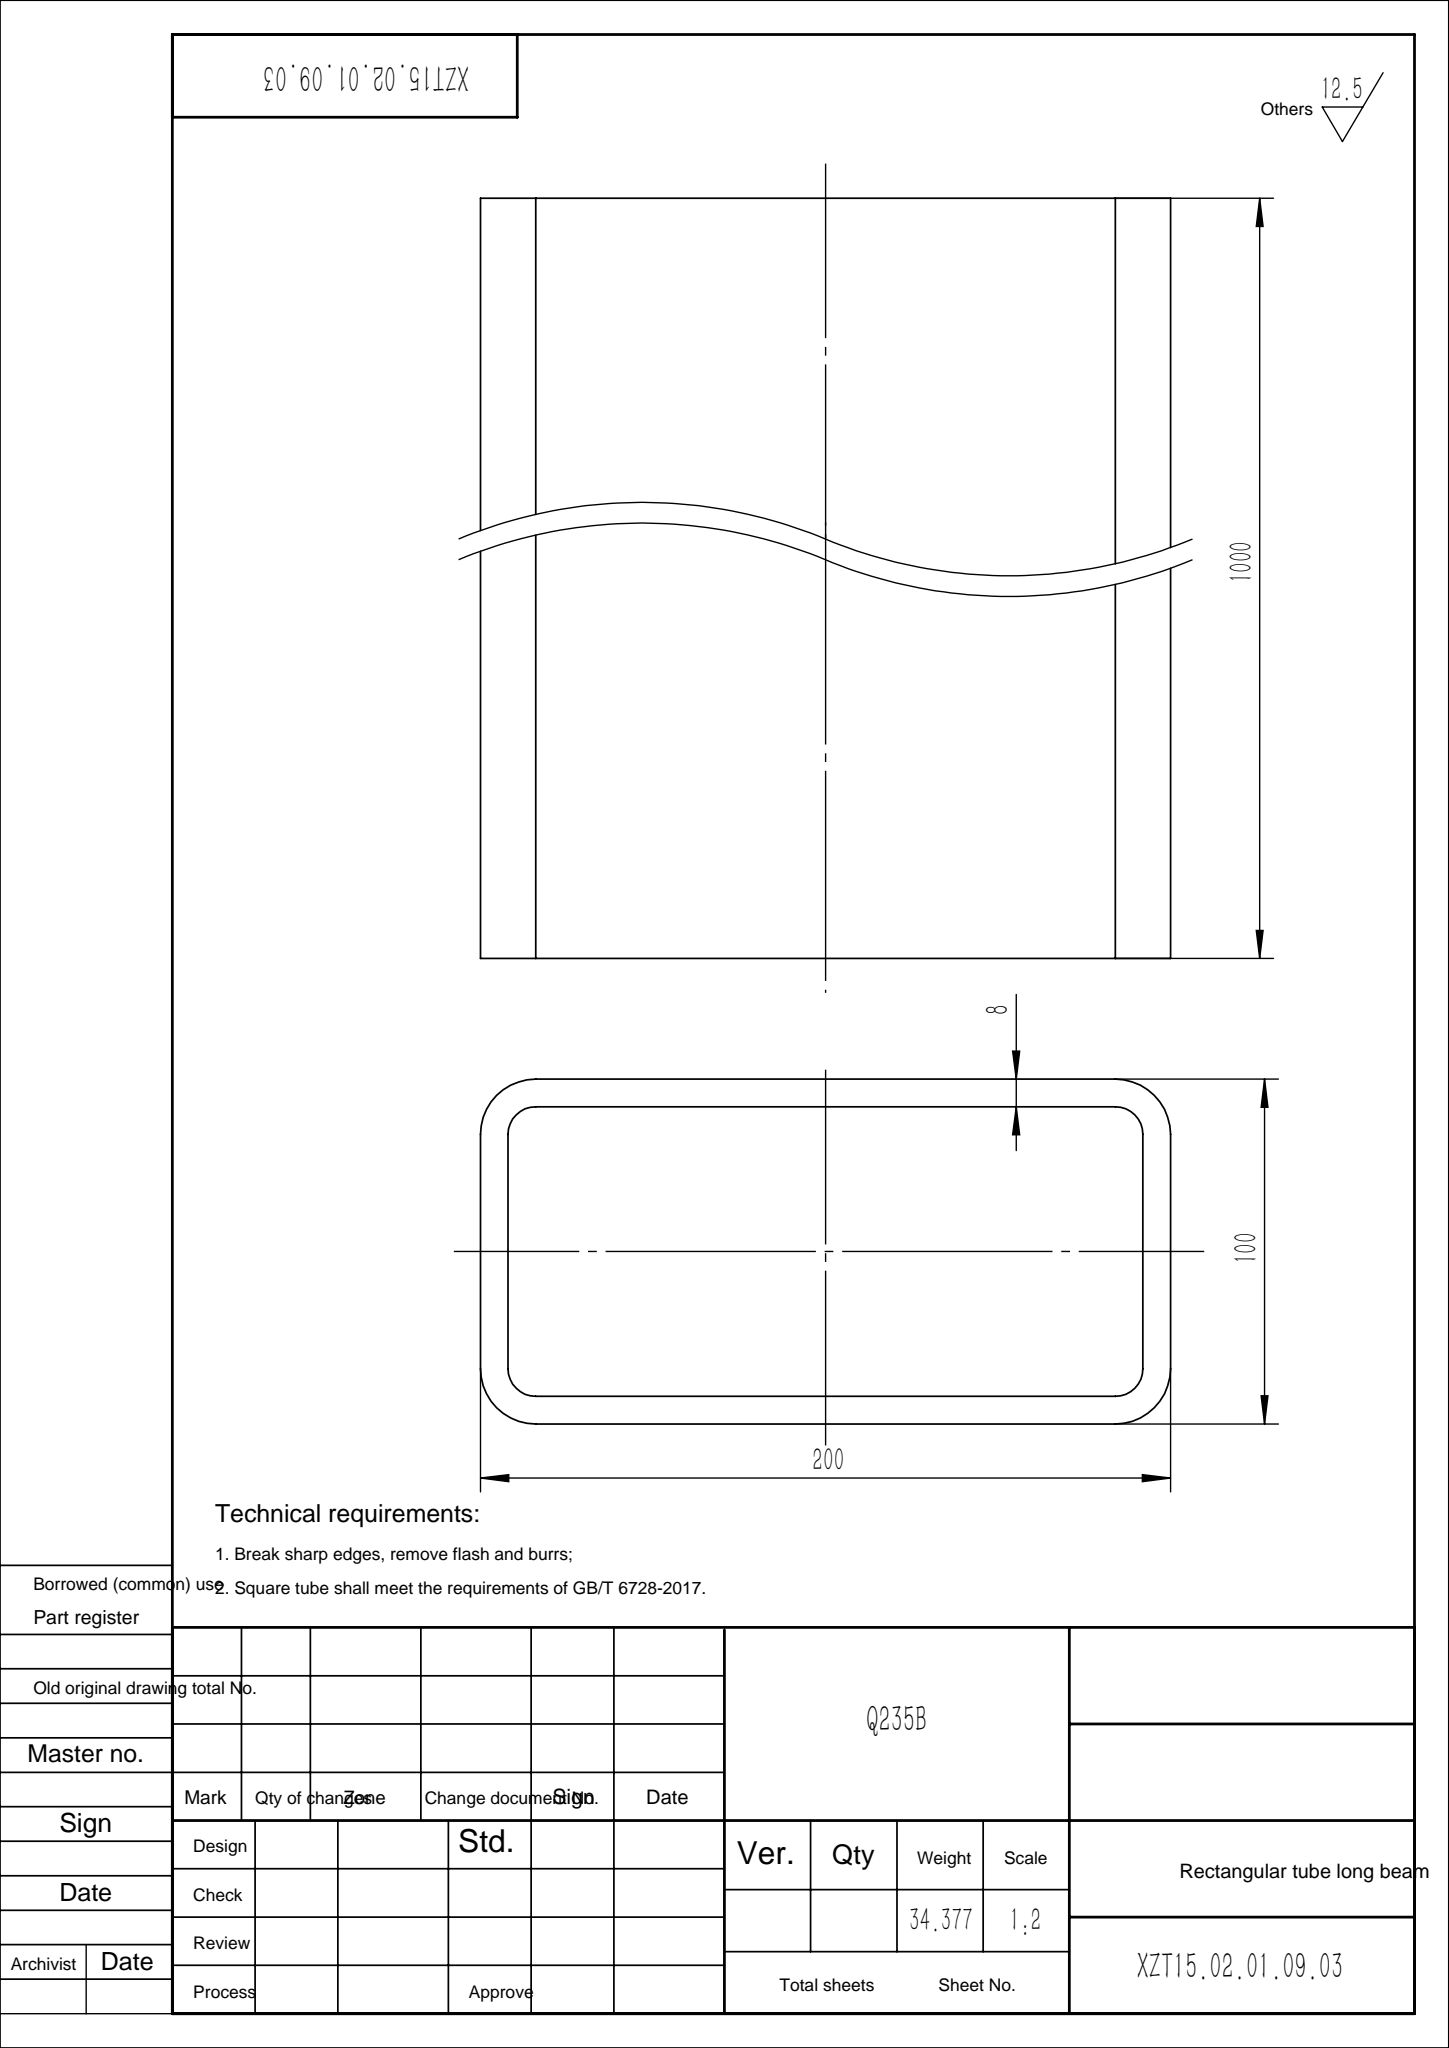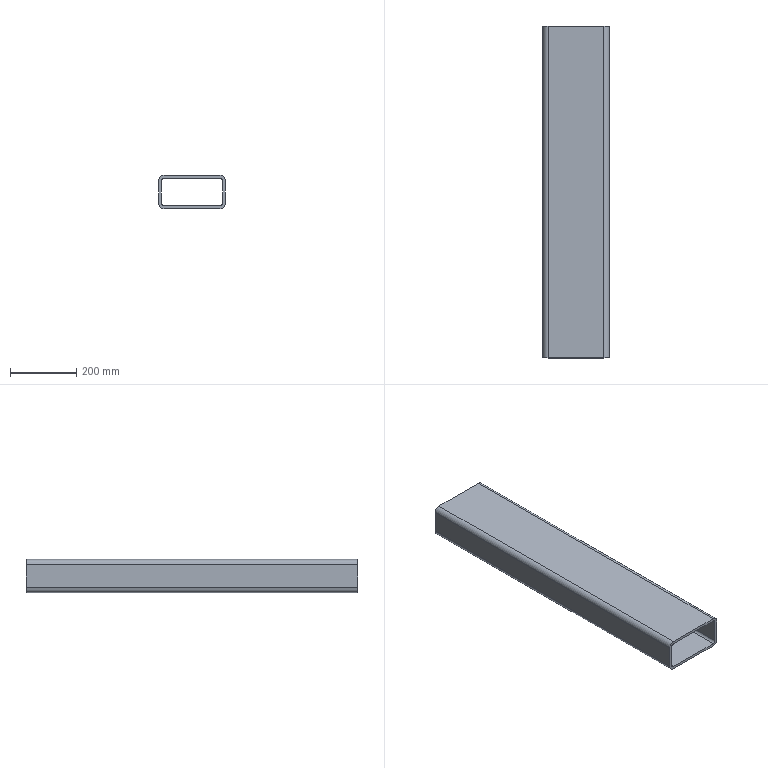Part | SolidWorks | features WeldMemberFeat 1, WeldmentFeature 1 | 1 solid | 18 faces | box 200 x 1000 x 100 mm | volume 4379186 mm3 | plane 10 | cylinder 8 | commonest cylinder face diameters 16 x4 32 x4
STEP:
#1=CARTESIAN_POINT('',(84.,0.,50.));
#2=VERTEX_POINT('',#1);
#3=CARTESIAN_POINT('',(100.,0.,34.));
#4=VERTEX_POINT('',#3);
#5=CARTESIAN_POINT('',(84.,0.,34.));
#6=DIRECTION('',(0.,1.,0.));
#7=DIRECTION('',(0.,0.,1.));
#8=AXIS2_PLACEMENT_3D('',#5,#6,#7);
#9=CIRCLE('',#8,16.);
#10=EDGE_CURVE('',#2,#4,#9,.T.);
#11=ORIENTED_EDGE('',*,*,#10,.T.);
#12=CARTESIAN_POINT('',(100.,1000.,34.));
#13=VERTEX_POINT('',#12);
#14=CARTESIAN_POINT('',(100.,1000.,34.));
#15=DIRECTION('',(0.,-1.,0.));
#16=VECTOR('',#15,1000.);
#17=LINE('',#14,#16);
#18=EDGE_CURVE('',#13,#4,#17,.T.);
#19=ORIENTED_EDGE('',*,*,#18,.F.);
#20=CARTESIAN_POINT('',(84.,1000.,50.));
#21=VERTEX_POINT('',#20);
#22=CARTESIAN_POINT('',(84.,1000.,34.));
#23=DIRECTION('',(0.,1.,0.));
#24=DIRECTION('',(0.,0.,1.));
#25=AXIS2_PLACEMENT_3D('',#22,#23,#24);
#26=CIRCLE('',#25,16.);
#27=EDGE_CURVE('',#21,#13,#26,.T.);
#28=ORIENTED_EDGE('',*,*,#27,.F.);
#29=CARTESIAN_POINT('',(84.,1000.,50.));
#30=DIRECTION('',(0.,-1.,0.));
#31=VECTOR('',#30,1000.);
#32=LINE('',#29,#31);
#33=EDGE_CURVE('',#21,#2,#32,.T.);
#34=ORIENTED_EDGE('',*,*,#33,.T.);
#35=EDGE_LOOP('',(#11,#19,#28,#34));
#36=FACE_OUTER_BOUND('',#35,.T.);
#37=CARTESIAN_POINT('',(84.,1000.,34.));
#38=DIRECTION('',(0.,-1.,0.));
#39=DIRECTION('',(0.,0.,-1.));
#40=AXIS2_PLACEMENT_3D('',#37,#38,#39);
#41=CYLINDRICAL_SURFACE('',#40,16.);
#42=ADVANCED_FACE('',(#36),#41,.T.);
#43=CARTESIAN_POINT('',(100.,0.,-34.));
#44=VERTEX_POINT('',#43);
#45=CARTESIAN_POINT('',(100.,0.,34.));
#46=DIRECTION('',(0.,0.,-1.));
#47=VECTOR('',#46,1000.);
#48=LINE('',#45,#47);
#49=EDGE_CURVE('',#4,#44,#48,.T.);
#50=ORIENTED_EDGE('',*,*,#49,.T.);
#51=CARTESIAN_POINT('',(100.,1000.,-34.));
#52=VERTEX_POINT('',#51);
#53=CARTESIAN_POINT('',(100.,1000.,-34.));
#54=DIRECTION('',(0.,-1.,0.));
#55=VECTOR('',#54,1000.);
#56=LINE('',#53,#55);
#57=EDGE_CURVE('',#52,#44,#56,.T.);
#58=ORIENTED_EDGE('',*,*,#57,.F.);
#59=CARTESIAN_POINT('',(100.,1000.,34.));
#60=DIRECTION('',(0.,0.,-1.));
#61=VECTOR('',#60,1000.);
#62=LINE('',#59,#61);
#63=EDGE_CURVE('',#13,#52,#62,.T.);
#64=ORIENTED_EDGE('',*,*,#63,.F.);
#65=ORIENTED_EDGE('',*,*,#18,.T.);
#66=EDGE_LOOP('',(#50,#58,#64,#65));
#67=FACE_OUTER_BOUND('',#66,.T.);
#68=CARTESIAN_POINT('',(100.,1000.,34.));
#69=DIRECTION('',(-1.,0.,0.));
#70=DIRECTION('',(0.,0.,1.));
#71=AXIS2_PLACEMENT_3D('',#68,#69,#70);
#72=PLANE('',#71);
#73=ADVANCED_FACE('',(#67),#72,.F.);
#74=CARTESIAN_POINT('',(84.,0.,-50.));
#75=VERTEX_POINT('',#74);
#76=CARTESIAN_POINT('',(84.,0.,-34.));
#77=DIRECTION('',(0.,1.,0.));
#78=DIRECTION('',(0.,0.,1.));
#79=AXIS2_PLACEMENT_3D('',#76,#77,#78);
#80=CIRCLE('',#79,16.);
#81=EDGE_CURVE('',#44,#75,#80,.T.);
#82=ORIENTED_EDGE('',*,*,#81,.T.);
#83=CARTESIAN_POINT('',(84.,1000.,-50.));
#84=VERTEX_POINT('',#83);
#85=CARTESIAN_POINT('',(84.,1000.,-50.));
#86=DIRECTION('',(0.,-1.,0.));
#87=VECTOR('',#86,1000.);
#88=LINE('',#85,#87);
#89=EDGE_CURVE('',#84,#75,#88,.T.);
#90=ORIENTED_EDGE('',*,*,#89,.F.);
#91=CARTESIAN_POINT('',(84.,1000.,-34.));
#92=DIRECTION('',(0.,1.,0.));
#93=DIRECTION('',(0.,0.,1.));
#94=AXIS2_PLACEMENT_3D('',#91,#92,#93);
#95=CIRCLE('',#94,16.);
#96=EDGE_CURVE('',#52,#84,#95,.T.);
#97=ORIENTED_EDGE('',*,*,#96,.F.);
#98=ORIENTED_EDGE('',*,*,#57,.T.);
#99=EDGE_LOOP('',(#82,#90,#97,#98));
#100=FACE_OUTER_BOUND('',#99,.T.);
#101=CARTESIAN_POINT('',(84.,1000.,-34.));
#102=DIRECTION('',(0.,-1.,0.));
#103=DIRECTION('',(0.,0.,-1.));
#104=AXIS2_PLACEMENT_3D('',#101,#102,#103);
#105=CYLINDRICAL_SURFACE('',#104,16.);
#106=ADVANCED_FACE('',(#100),#105,.T.);
#107=CARTESIAN_POINT('',(-84.,0.,-50.));
#108=VERTEX_POINT('',#107);
#109=CARTESIAN_POINT('',(-84.,0.,-50.));
#110=DIRECTION('',(-1.,0.,0.));
#111=VECTOR('',#110,1000.);
#112=LINE('',#109,#111);
#113=EDGE_CURVE('',#75,#108,#112,.T.);
#114=ORIENTED_EDGE('',*,*,#113,.T.);
#115=CARTESIAN_POINT('',(-84.,1000.,-50.));
#116=VERTEX_POINT('',#115);
#117=CARTESIAN_POINT('',(-84.,1000.,-50.));
#118=DIRECTION('',(0.,-1.,0.));
#119=VECTOR('',#118,1000.);
#120=LINE('',#117,#119);
#121=EDGE_CURVE('',#116,#108,#120,.T.);
#122=ORIENTED_EDGE('',*,*,#121,.F.);
#123=CARTESIAN_POINT('',(-84.,1000.,-50.));
#124=DIRECTION('',(-1.,0.,0.));
#125=VECTOR('',#124,1000.);
#126=LINE('',#123,#125);
#127=EDGE_CURVE('',#84,#116,#126,.T.);
#128=ORIENTED_EDGE('',*,*,#127,.F.);
#129=ORIENTED_EDGE('',*,*,#89,.T.);
#130=EDGE_LOOP('',(#114,#122,#128,#129));
#131=FACE_OUTER_BOUND('',#130,.T.);
#132=CARTESIAN_POINT('',(-84.,1000.,-50.));
#133=DIRECTION('',(0.,0.,1.));
#134=DIRECTION('',(1.,0.,0.));
#135=AXIS2_PLACEMENT_3D('',#132,#133,#134);
#136=PLANE('',#135);
#137=ADVANCED_FACE('',(#131),#136,.F.);
#138=CARTESIAN_POINT('',(-100.,0.,-34.));
#139=VERTEX_POINT('',#138);
#140=CARTESIAN_POINT('',(-84.,0.,-34.));
#141=DIRECTION('',(0.,1.,0.));
#142=DIRECTION('',(0.,0.,1.));
#143=AXIS2_PLACEMENT_3D('',#140,#141,#142);
#144=CIRCLE('',#143,16.);
#145=EDGE_CURVE('',#108,#139,#144,.T.);
#146=ORIENTED_EDGE('',*,*,#145,.T.);
#147=CARTESIAN_POINT('',(-100.,1000.,-34.));
#148=VERTEX_POINT('',#147);
#149=CARTESIAN_POINT('',(-100.,1000.,-34.));
#150=DIRECTION('',(0.,-1.,0.));
#151=VECTOR('',#150,1000.);
#152=LINE('',#149,#151);
#153=EDGE_CURVE('',#148,#139,#152,.T.);
#154=ORIENTED_EDGE('',*,*,#153,.F.);
#155=CARTESIAN_POINT('',(-84.,1000.,-34.));
#156=DIRECTION('',(0.,1.,0.));
#157=DIRECTION('',(0.,0.,1.));
#158=AXIS2_PLACEMENT_3D('',#155,#156,#157);
#159=CIRCLE('',#158,16.);
#160=EDGE_CURVE('',#116,#148,#159,.T.);
#161=ORIENTED_EDGE('',*,*,#160,.F.);
#162=ORIENTED_EDGE('',*,*,#121,.T.);
#163=EDGE_LOOP('',(#146,#154,#161,#162));
#164=FACE_OUTER_BOUND('',#163,.T.);
#165=CARTESIAN_POINT('',(-84.,1000.,-34.));
#166=DIRECTION('',(0.,-1.,0.));
#167=DIRECTION('',(0.,0.,-1.));
#168=AXIS2_PLACEMENT_3D('',#165,#166,#167);
#169=CYLINDRICAL_SURFACE('',#168,16.);
#170=ADVANCED_FACE('',(#164),#169,.T.);
#171=CARTESIAN_POINT('',(-100.,0.,34.));
#172=VERTEX_POINT('',#171);
#173=CARTESIAN_POINT('',(-100.,0.,-34.));
#174=DIRECTION('',(0.,0.,1.));
#175=VECTOR('',#174,1000.);
#176=LINE('',#173,#175);
#177=EDGE_CURVE('',#139,#172,#176,.T.);
#178=ORIENTED_EDGE('',*,*,#177,.T.);
#179=CARTESIAN_POINT('',(-100.,1000.,34.));
#180=VERTEX_POINT('',#179);
#181=CARTESIAN_POINT('',(-100.,1000.,34.));
#182=DIRECTION('',(0.,-1.,0.));
#183=VECTOR('',#182,1000.);
#184=LINE('',#181,#183);
#185=EDGE_CURVE('',#180,#172,#184,.T.);
#186=ORIENTED_EDGE('',*,*,#185,.F.);
#187=CARTESIAN_POINT('',(-100.,1000.,-34.));
#188=DIRECTION('',(0.,0.,1.));
#189=VECTOR('',#188,1000.);
#190=LINE('',#187,#189);
#191=EDGE_CURVE('',#148,#180,#190,.T.);
#192=ORIENTED_EDGE('',*,*,#191,.F.);
#193=ORIENTED_EDGE('',*,*,#153,.T.);
#194=EDGE_LOOP('',(#178,#186,#192,#193));
#195=FACE_OUTER_BOUND('',#194,.T.);
#196=CARTESIAN_POINT('',(-100.,1000.,-34.));
#197=DIRECTION('',(1.,0.,0.));
#198=DIRECTION('',(0.,0.,-1.));
#199=AXIS2_PLACEMENT_3D('',#196,#197,#198);
#200=PLANE('',#199);
#201=ADVANCED_FACE('',(#195),#200,.F.);
#202=CARTESIAN_POINT('',(-84.,0.,50.));
#203=VERTEX_POINT('',#202);
#204=CARTESIAN_POINT('',(-84.,0.,34.));
#205=DIRECTION('',(0.,1.,0.));
#206=DIRECTION('',(0.,0.,1.));
#207=AXIS2_PLACEMENT_3D('',#204,#205,#206);
#208=CIRCLE('',#207,16.);
#209=EDGE_CURVE('',#172,#203,#208,.T.);
#210=ORIENTED_EDGE('',*,*,#209,.T.);
#211=CARTESIAN_POINT('',(-84.,1000.,50.));
#212=VERTEX_POINT('',#211);
#213=CARTESIAN_POINT('',(-84.,1000.,50.));
#214=DIRECTION('',(0.,-1.,0.));
#215=VECTOR('',#214,1000.);
#216=LINE('',#213,#215);
#217=EDGE_CURVE('',#212,#203,#216,.T.);
#218=ORIENTED_EDGE('',*,*,#217,.F.);
#219=CARTESIAN_POINT('',(-84.,1000.,34.));
#220=DIRECTION('',(0.,1.,0.));
#221=DIRECTION('',(0.,0.,1.));
#222=AXIS2_PLACEMENT_3D('',#219,#220,#221);
#223=CIRCLE('',#222,16.);
#224=EDGE_CURVE('',#180,#212,#223,.T.);
#225=ORIENTED_EDGE('',*,*,#224,.F.);
#226=ORIENTED_EDGE('',*,*,#185,.T.);
#227=EDGE_LOOP('',(#210,#218,#225,#226));
#228=FACE_OUTER_BOUND('',#227,.T.);
#229=CARTESIAN_POINT('',(-84.,1000.,34.));
#230=DIRECTION('',(0.,-1.,0.));
#231=DIRECTION('',(0.,0.,-1.));
#232=AXIS2_PLACEMENT_3D('',#229,#230,#231);
#233=CYLINDRICAL_SURFACE('',#232,16.);
#234=ADVANCED_FACE('',(#228),#233,.T.);
#235=CARTESIAN_POINT('',(92.,0.,-34.));
#236=VERTEX_POINT('',#235);
#237=CARTESIAN_POINT('',(84.,0.,-42.));
#238=VERTEX_POINT('',#237);
#239=CARTESIAN_POINT('',(84.,0.,-34.));
#240=DIRECTION('',(0.,1.,0.));
#241=DIRECTION('',(0.,0.,1.));
#242=AXIS2_PLACEMENT_3D('',#239,#240,#241);
#243=CIRCLE('',#242,8.);
#244=EDGE_CURVE('',#236,#238,#243,.T.);
#245=ORIENTED_EDGE('',*,*,#244,.F.);
#246=CARTESIAN_POINT('',(92.,1000.,-34.));
#247=VERTEX_POINT('',#246);
#248=CARTESIAN_POINT('',(92.,1000.,-34.));
#249=DIRECTION('',(0.,-1.,0.));
#250=VECTOR('',#249,1000.);
#251=LINE('',#248,#250);
#252=EDGE_CURVE('',#247,#236,#251,.T.);
#253=ORIENTED_EDGE('',*,*,#252,.F.);
#254=CARTESIAN_POINT('',(84.,1000.,-42.));
#255=VERTEX_POINT('',#254);
#256=CARTESIAN_POINT('',(84.,1000.,-34.));
#257=DIRECTION('',(0.,1.,0.));
#258=DIRECTION('',(0.,0.,1.));
#259=AXIS2_PLACEMENT_3D('',#256,#257,#258);
#260=CIRCLE('',#259,8.);
#261=EDGE_CURVE('',#247,#255,#260,.T.);
#262=ORIENTED_EDGE('',*,*,#261,.T.);
#263=CARTESIAN_POINT('',(84.,1000.,-42.));
#264=DIRECTION('',(0.,-1.,0.));
#265=VECTOR('',#264,1000.);
#266=LINE('',#263,#265);
#267=EDGE_CURVE('',#255,#238,#266,.T.);
#268=ORIENTED_EDGE('',*,*,#267,.T.);
#269=EDGE_LOOP('',(#245,#253,#262,#268));
#270=FACE_OUTER_BOUND('',#269,.T.);
#271=CARTESIAN_POINT('',(84.,1000.,-34.));
#272=DIRECTION('',(0.,-1.,0.));
#273=DIRECTION('',(0.,0.,-1.));
#274=AXIS2_PLACEMENT_3D('',#271,#272,#273);
#275=CYLINDRICAL_SURFACE('',#274,8.);
#276=ADVANCED_FACE('',(#270),#275,.F.);
#277=CARTESIAN_POINT('',(92.,0.,34.));
#278=VERTEX_POINT('',#277);
#279=CARTESIAN_POINT('',(92.,0.,34.));
#280=DIRECTION('',(0.,0.,-1.));
#281=VECTOR('',#280,1000.);
#282=LINE('',#279,#281);
#283=EDGE_CURVE('',#278,#236,#282,.T.);
#284=ORIENTED_EDGE('',*,*,#283,.F.);
#285=CARTESIAN_POINT('',(92.,1000.,34.));
#286=VERTEX_POINT('',#285);
#287=CARTESIAN_POINT('',(92.,1000.,34.));
#288=DIRECTION('',(0.,-1.,0.));
#289=VECTOR('',#288,1000.);
#290=LINE('',#287,#289);
#291=EDGE_CURVE('',#286,#278,#290,.T.);
#292=ORIENTED_EDGE('',*,*,#291,.F.);
#293=CARTESIAN_POINT('',(92.,1000.,34.));
#294=DIRECTION('',(0.,0.,-1.));
#295=VECTOR('',#294,1000.);
#296=LINE('',#293,#295);
#297=EDGE_CURVE('',#286,#247,#296,.T.);
#298=ORIENTED_EDGE('',*,*,#297,.T.);
#299=ORIENTED_EDGE('',*,*,#252,.T.);
#300=EDGE_LOOP('',(#284,#292,#298,#299));
#301=FACE_OUTER_BOUND('',#300,.T.);
#302=CARTESIAN_POINT('',(92.,1000.,34.));
#303=DIRECTION('',(-1.,0.,0.));
#304=DIRECTION('',(0.,0.,1.));
#305=AXIS2_PLACEMENT_3D('',#302,#303,#304);
#306=PLANE('',#305);
#307=ADVANCED_FACE('',(#301),#306,.T.);
#308=CARTESIAN_POINT('',(84.,0.,42.));
#309=VERTEX_POINT('',#308);
#310=CARTESIAN_POINT('',(84.,0.,34.));
#311=DIRECTION('',(0.,1.,0.));
#312=DIRECTION('',(0.,0.,1.));
#313=AXIS2_PLACEMENT_3D('',#310,#311,#312);
#314=CIRCLE('',#313,8.);
#315=EDGE_CURVE('',#309,#278,#314,.T.);
#316=ORIENTED_EDGE('',*,*,#315,.F.);
#317=CARTESIAN_POINT('',(84.,1000.,42.));
#318=VERTEX_POINT('',#317);
#319=CARTESIAN_POINT('',(84.,1000.,42.));
#320=DIRECTION('',(0.,-1.,0.));
#321=VECTOR('',#320,1000.);
#322=LINE('',#319,#321);
#323=EDGE_CURVE('',#318,#309,#322,.T.);
#324=ORIENTED_EDGE('',*,*,#323,.F.);
#325=CARTESIAN_POINT('',(84.,1000.,34.));
#326=DIRECTION('',(0.,1.,0.));
#327=DIRECTION('',(0.,0.,1.));
#328=AXIS2_PLACEMENT_3D('',#325,#326,#327);
#329=CIRCLE('',#328,8.);
#330=EDGE_CURVE('',#318,#286,#329,.T.);
#331=ORIENTED_EDGE('',*,*,#330,.T.);
#332=ORIENTED_EDGE('',*,*,#291,.T.);
#333=EDGE_LOOP('',(#316,#324,#331,#332));
#334=FACE_OUTER_BOUND('',#333,.T.);
#335=CARTESIAN_POINT('',(84.,1000.,34.));
#336=DIRECTION('',(0.,-1.,0.));
#337=DIRECTION('',(0.,0.,-1.));
#338=AXIS2_PLACEMENT_3D('',#335,#336,#337);
#339=CYLINDRICAL_SURFACE('',#338,8.);
#340=ADVANCED_FACE('',(#334),#339,.F.);
#341=CARTESIAN_POINT('',(-84.,0.,42.));
#342=VERTEX_POINT('',#341);
#343=CARTESIAN_POINT('',(84.,0.,42.));
#344=DIRECTION('',(1.,0.,0.));
#345=VECTOR('',#344,1000.);
#346=LINE('',#343,#345);
#347=EDGE_CURVE('',#342,#309,#346,.T.);
#348=ORIENTED_EDGE('',*,*,#347,.F.);
#349=CARTESIAN_POINT('',(-84.,1000.,42.));
#350=VERTEX_POINT('',#349);
#351=CARTESIAN_POINT('',(-84.,1000.,42.));
#352=DIRECTION('',(0.,-1.,0.));
#353=VECTOR('',#352,1000.);
#354=LINE('',#351,#353);
#355=EDGE_CURVE('',#350,#342,#354,.T.);
#356=ORIENTED_EDGE('',*,*,#355,.F.);
#357=CARTESIAN_POINT('',(84.,1000.,42.));
#358=DIRECTION('',(1.,0.,0.));
#359=VECTOR('',#358,1000.);
#360=LINE('',#357,#359);
#361=EDGE_CURVE('',#350,#318,#360,.T.);
#362=ORIENTED_EDGE('',*,*,#361,.T.);
#363=ORIENTED_EDGE('',*,*,#323,.T.);
#364=EDGE_LOOP('',(#348,#356,#362,#363));
#365=FACE_OUTER_BOUND('',#364,.T.);
#366=CARTESIAN_POINT('',(84.,1000.,42.));
#367=DIRECTION('',(0.,0.,-1.));
#368=DIRECTION('',(-1.,0.,0.));
#369=AXIS2_PLACEMENT_3D('',#366,#367,#368);
#370=PLANE('',#369);
#371=ADVANCED_FACE('',(#365),#370,.T.);
#372=CARTESIAN_POINT('',(-92.,0.,34.));
#373=VERTEX_POINT('',#372);
#374=CARTESIAN_POINT('',(-84.,0.,34.));
#375=DIRECTION('',(0.,1.,0.));
#376=DIRECTION('',(0.,0.,1.));
#377=AXIS2_PLACEMENT_3D('',#374,#375,#376);
#378=CIRCLE('',#377,8.);
#379=EDGE_CURVE('',#373,#342,#378,.T.);
#380=ORIENTED_EDGE('',*,*,#379,.F.);
#381=CARTESIAN_POINT('',(-92.,1000.,34.));
#382=VERTEX_POINT('',#381);
#383=CARTESIAN_POINT('',(-92.,1000.,34.));
#384=DIRECTION('',(0.,-1.,0.));
#385=VECTOR('',#384,1000.);
#386=LINE('',#383,#385);
#387=EDGE_CURVE('',#382,#373,#386,.T.);
#388=ORIENTED_EDGE('',*,*,#387,.F.);
#389=CARTESIAN_POINT('',(-84.,1000.,34.));
#390=DIRECTION('',(0.,1.,0.));
#391=DIRECTION('',(0.,0.,1.));
#392=AXIS2_PLACEMENT_3D('',#389,#390,#391);
#393=CIRCLE('',#392,8.);
#394=EDGE_CURVE('',#382,#350,#393,.T.);
#395=ORIENTED_EDGE('',*,*,#394,.T.);
#396=ORIENTED_EDGE('',*,*,#355,.T.);
#397=EDGE_LOOP('',(#380,#388,#395,#396));
#398=FACE_OUTER_BOUND('',#397,.T.);
#399=CARTESIAN_POINT('',(-84.,1000.,34.));
#400=DIRECTION('',(0.,-1.,0.));
#401=DIRECTION('',(0.,0.,-1.));
#402=AXIS2_PLACEMENT_3D('',#399,#400,#401);
#403=CYLINDRICAL_SURFACE('',#402,8.);
#404=ADVANCED_FACE('',(#398),#403,.F.);
#405=CARTESIAN_POINT('',(-92.,0.,-34.));
#406=VERTEX_POINT('',#405);
#407=CARTESIAN_POINT('',(-92.,0.,-34.));
#408=DIRECTION('',(0.,0.,1.));
#409=VECTOR('',#408,1000.);
#410=LINE('',#407,#409);
#411=EDGE_CURVE('',#406,#373,#410,.T.);
#412=ORIENTED_EDGE('',*,*,#411,.F.);
#413=CARTESIAN_POINT('',(-92.,1000.,-34.));
#414=VERTEX_POINT('',#413);
#415=CARTESIAN_POINT('',(-92.,1000.,-34.));
#416=DIRECTION('',(0.,-1.,0.));
#417=VECTOR('',#416,1000.);
#418=LINE('',#415,#417);
#419=EDGE_CURVE('',#414,#406,#418,.T.);
#420=ORIENTED_EDGE('',*,*,#419,.F.);
#421=CARTESIAN_POINT('',(-92.,1000.,-34.));
#422=DIRECTION('',(0.,0.,1.));
#423=VECTOR('',#422,1000.);
#424=LINE('',#421,#423);
#425=EDGE_CURVE('',#414,#382,#424,.T.);
#426=ORIENTED_EDGE('',*,*,#425,.T.);
#427=ORIENTED_EDGE('',*,*,#387,.T.);
#428=EDGE_LOOP('',(#412,#420,#426,#427));
#429=FACE_OUTER_BOUND('',#428,.T.);
#430=CARTESIAN_POINT('',(-92.,1000.,-34.));
#431=DIRECTION('',(1.,0.,0.));
#432=DIRECTION('',(0.,0.,-1.));
#433=AXIS2_PLACEMENT_3D('',#430,#431,#432);
#434=PLANE('',#433);
#435=ADVANCED_FACE('',(#429),#434,.T.);
#436=CARTESIAN_POINT('',(-84.,0.,-42.));
#437=VERTEX_POINT('',#436);
#438=CARTESIAN_POINT('',(-84.,0.,-34.));
#439=DIRECTION('',(0.,1.,0.));
#440=DIRECTION('',(0.,0.,1.));
#441=AXIS2_PLACEMENT_3D('',#438,#439,#440);
#442=CIRCLE('',#441,8.);
#443=EDGE_CURVE('',#437,#406,#442,.T.);
#444=ORIENTED_EDGE('',*,*,#443,.F.);
#445=CARTESIAN_POINT('',(-84.,1000.,-42.));
#446=VERTEX_POINT('',#445);
#447=CARTESIAN_POINT('',(-84.,1000.,-42.));
#448=DIRECTION('',(0.,-1.,0.));
#449=VECTOR('',#448,1000.);
#450=LINE('',#447,#449);
#451=EDGE_CURVE('',#446,#437,#450,.T.);
#452=ORIENTED_EDGE('',*,*,#451,.F.);
#453=CARTESIAN_POINT('',(-84.,1000.,-34.));
#454=DIRECTION('',(0.,1.,0.));
#455=DIRECTION('',(0.,0.,1.));
#456=AXIS2_PLACEMENT_3D('',#453,#454,#455);
#457=CIRCLE('',#456,8.);
#458=EDGE_CURVE('',#446,#414,#457,.T.);
#459=ORIENTED_EDGE('',*,*,#458,.T.);
#460=ORIENTED_EDGE('',*,*,#419,.T.);
#461=EDGE_LOOP('',(#444,#452,#459,#460));
#462=FACE_OUTER_BOUND('',#461,.T.);
#463=CARTESIAN_POINT('',(-84.,1000.,-34.));
#464=DIRECTION('',(0.,-1.,0.));
#465=DIRECTION('',(0.,0.,-1.));
#466=AXIS2_PLACEMENT_3D('',#463,#464,#465);
#467=CYLINDRICAL_SURFACE('',#466,8.);
#468=ADVANCED_FACE('',(#462),#467,.F.);
#469=CARTESIAN_POINT('',(-84.,0.,-42.));
#470=DIRECTION('',(-1.,0.,0.));
#471=VECTOR('',#470,1000.);
#472=LINE('',#469,#471);
#473=EDGE_CURVE('',#238,#437,#472,.T.);
#474=ORIENTED_EDGE('',*,*,#473,.F.);
#475=ORIENTED_EDGE('',*,*,#267,.F.);
#476=CARTESIAN_POINT('',(-84.,1000.,-42.));
#477=DIRECTION('',(-1.,0.,0.));
#478=VECTOR('',#477,1000.);
#479=LINE('',#476,#478);
#480=EDGE_CURVE('',#255,#446,#479,.T.);
#481=ORIENTED_EDGE('',*,*,#480,.T.);
#482=ORIENTED_EDGE('',*,*,#451,.T.);
#483=EDGE_LOOP('',(#474,#475,#481,#482));
#484=FACE_OUTER_BOUND('',#483,.T.);
#485=CARTESIAN_POINT('',(-84.,1000.,-42.));
#486=DIRECTION('',(0.,0.,1.));
#487=DIRECTION('',(1.,0.,0.));
#488=AXIS2_PLACEMENT_3D('',#485,#486,#487);
#489=PLANE('',#488);
#490=ADVANCED_FACE('',(#484),#489,.T.);
#491=CARTESIAN_POINT('',(84.,0.,50.));
#492=DIRECTION('',(1.,0.,0.));
#493=VECTOR('',#492,1000.);
#494=LINE('',#491,#493);
#495=EDGE_CURVE('',#203,#2,#494,.T.);
#496=ORIENTED_EDGE('',*,*,#495,.T.);
#497=ORIENTED_EDGE('',*,*,#33,.F.);
#498=CARTESIAN_POINT('',(84.,1000.,50.));
#499=DIRECTION('',(1.,0.,0.));
#500=VECTOR('',#499,1000.);
#501=LINE('',#498,#500);
#502=EDGE_CURVE('',#212,#21,#501,.T.);
#503=ORIENTED_EDGE('',*,*,#502,.F.);
#504=ORIENTED_EDGE('',*,*,#217,.T.);
#505=EDGE_LOOP('',(#496,#497,#503,#504));
#506=FACE_OUTER_BOUND('',#505,.T.);
#507=CARTESIAN_POINT('',(84.,1000.,50.));
#508=DIRECTION('',(0.,0.,-1.));
#509=DIRECTION('',(-1.,0.,0.));
#510=AXIS2_PLACEMENT_3D('',#507,#508,#509);
#511=PLANE('',#510);
#512=ADVANCED_FACE('',(#506),#511,.F.);
#513=ORIENTED_EDGE('',*,*,#261,.F.);
#514=ORIENTED_EDGE('',*,*,#297,.F.);
#515=ORIENTED_EDGE('',*,*,#330,.F.);
#516=ORIENTED_EDGE('',*,*,#361,.F.);
#517=ORIENTED_EDGE('',*,*,#394,.F.);
#518=ORIENTED_EDGE('',*,*,#425,.F.);
#519=ORIENTED_EDGE('',*,*,#458,.F.);
#520=ORIENTED_EDGE('',*,*,#480,.F.);
#521=EDGE_LOOP('',(#513,#514,#515,#516,#517,#518,#519,#520));
#522=FACE_BOUND('',#521,.T.);
#523=ORIENTED_EDGE('',*,*,#27,.T.);
#524=ORIENTED_EDGE('',*,*,#63,.T.);
#525=ORIENTED_EDGE('',*,*,#96,.T.);
#526=ORIENTED_EDGE('',*,*,#127,.T.);
#527=ORIENTED_EDGE('',*,*,#160,.T.);
#528=ORIENTED_EDGE('',*,*,#191,.T.);
#529=ORIENTED_EDGE('',*,*,#224,.T.);
#530=ORIENTED_EDGE('',*,*,#502,.T.);
#531=EDGE_LOOP('',(#523,#524,#525,#526,#527,#528,#529,#530));
#532=FACE_OUTER_BOUND('',#531,.T.);
#533=CARTESIAN_POINT('',(84.,1000.,34.));
#534=DIRECTION('',(0.,1.,0.));
#535=DIRECTION('',(0.,0.,1.));
#536=AXIS2_PLACEMENT_3D('',#533,#534,#535);
#537=PLANE('',#536);
#538=ADVANCED_FACE('',(#522,#532),#537,.T.);
#539=ORIENTED_EDGE('',*,*,#244,.T.);
#540=ORIENTED_EDGE('',*,*,#473,.T.);
#541=ORIENTED_EDGE('',*,*,#443,.T.);
#542=ORIENTED_EDGE('',*,*,#411,.T.);
#543=ORIENTED_EDGE('',*,*,#379,.T.);
#544=ORIENTED_EDGE('',*,*,#347,.T.);
#545=ORIENTED_EDGE('',*,*,#315,.T.);
#546=ORIENTED_EDGE('',*,*,#283,.T.);
#547=EDGE_LOOP('',(#539,#540,#541,#542,#543,#544,#545,#546));
#548=FACE_BOUND('',#547,.T.);
#549=ORIENTED_EDGE('',*,*,#10,.F.);
#550=ORIENTED_EDGE('',*,*,#495,.F.);
#551=ORIENTED_EDGE('',*,*,#209,.F.);
#552=ORIENTED_EDGE('',*,*,#177,.F.);
#553=ORIENTED_EDGE('',*,*,#145,.F.);
#554=ORIENTED_EDGE('',*,*,#113,.F.);
#555=ORIENTED_EDGE('',*,*,#81,.F.);
#556=ORIENTED_EDGE('',*,*,#49,.F.);
#557=EDGE_LOOP('',(#549,#550,#551,#552,#553,#554,#555,#556));
#558=FACE_OUTER_BOUND('',#557,.T.);
#559=CARTESIAN_POINT('',(84.,0.,34.));
#560=DIRECTION('',(0.,1.,0.));
#561=DIRECTION('',(0.,0.,1.));
#562=AXIS2_PLACEMENT_3D('',#559,#560,#561);
#563=PLANE('',#562);
#564=ADVANCED_FACE('',(#548,#558),#563,.F.);
#565=CLOSED_SHELL('',(#42,#73,#106,#137,#170,#201,#234,#276,#307,#340,#371,#404,#435,#468,#490,#512,#538,#564));
#566=MANIFOLD_SOLID_BREP('',#565);
#567=CARTESIAN_POINT('',(0.,0.,0.));
#568=DIRECTION('',(0.,0.,1.));
#569=DIRECTION('',(1.,0.,0.));
#570=AXIS2_PLACEMENT_3D('',#567,#568,#569);
#571=(LENGTH_UNIT()NAMED_UNIT(*)SI_UNIT(.MILLI.,.METRE.));
#572=UNCERTAINTY_MEASURE_WITH_UNIT(LENGTH_MEASURE(0.00001),#571,'','');
#573=(NAMED_UNIT(*)PLANE_ANGLE_UNIT()SI_UNIT($,.RADIAN.));
#574=(NAMED_UNIT(*)SI_UNIT($,.STERADIAN.)SOLID_ANGLE_UNIT());
#575=(GEOMETRIC_REPRESENTATION_CONTEXT(3)GLOBAL_UNCERTAINTY_ASSIGNED_CONTEXT((#572))GLOBAL_UNIT_ASSIGNED_CONTEXT((#571,#573,#574))REPRESENTATION_CONTEXT('',''));
#576=ADVANCED_BREP_SHAPE_REPRESENTATION('',(#566,#570),#575);